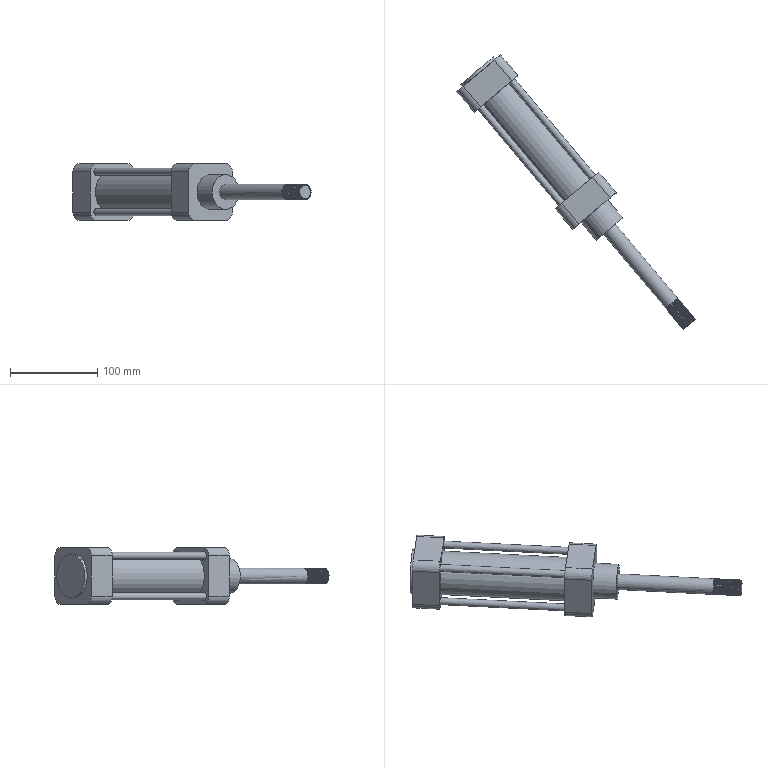Part | NX | features solid 2 | 1 solid | 71 faces | box 272.421 x 313.698 x 65 mm | volume 642187 mm3 | cylinder 45 | plane 24 | spline 2 | commonest cylinder face diameters 18 x21 18.5 x8 10 x6 8 x4 6.667 x2 50 x2